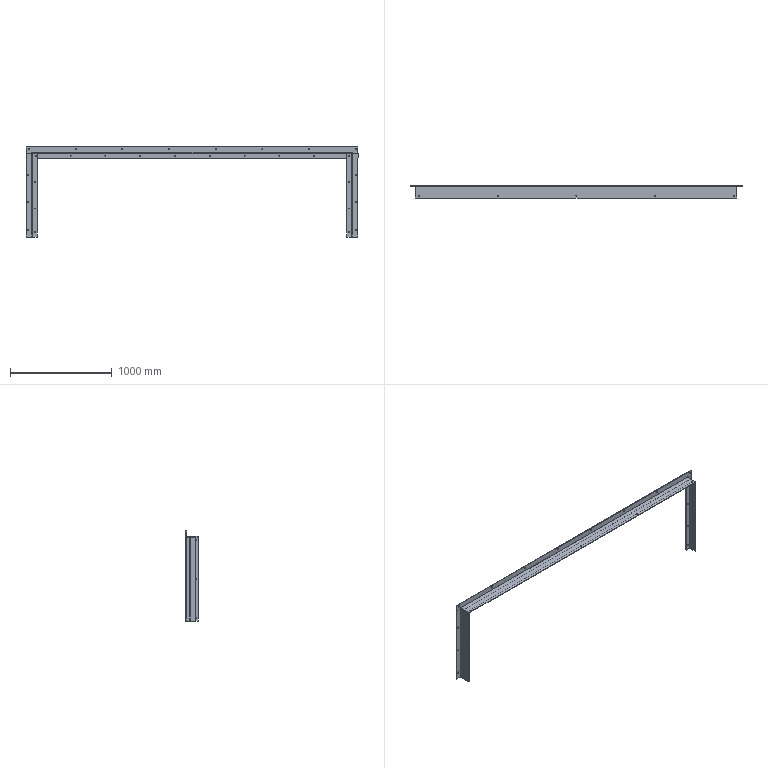Part | SolidWorks | 6 solids | 182 faces | box 3271 x 120 x 887 mm | volume 7624101 mm3 | cylinder 94 | plane 60 | cone 28 | commonest cylinder face diameters 9 x82 1.473 x6 13.473 x6